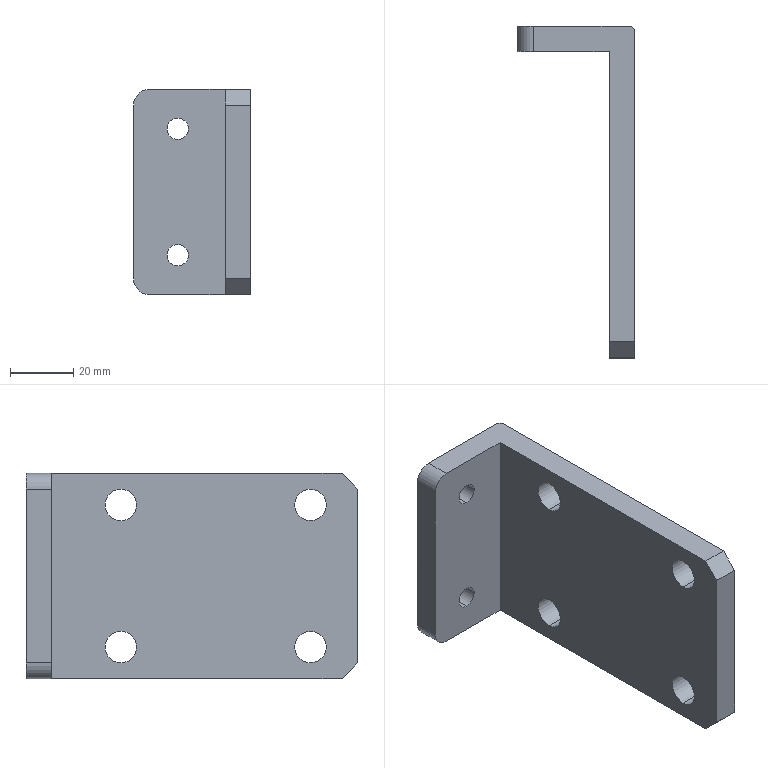Part | NX | features BREP 1 | 1 solid | 25 faces | box 37 x 105 x 65 mm | volume 66267 mm3 | cylinder 14 | plane 11 | commonest cylinder face diameters 10 x10 6.8 x4
STEP:
#1=CARTESIAN_POINT('',(0.,-30.,5.));
#2=VERTEX_POINT('',#1);
#3=CARTESIAN_POINT('',(0.,-30.,15.));
#4=VERTEX_POINT('',#3);
#5=CARTESIAN_POINT('',(0.,-30.,10.));
#6=DIRECTION('',(-1.,0.,0.));
#7=DIRECTION('',(0.,0.,1.));
#8=AXIS2_PLACEMENT_3D('',#5,#6,#7);
#9=CIRCLE('',#8,5.);
#10=EDGE_CURVE('',#2,#4,#9,.T.);
#11=ORIENTED_EDGE('',*,*,#10,.F.);
#12=CARTESIAN_POINT('',(-8.,-30.,5.));
#13=VERTEX_POINT('',#12);
#14=CARTESIAN_POINT('',(-8.,-30.,5.));
#15=DIRECTION('',(-1.,0.,0.));
#16=VECTOR('',#15,1000.);
#17=LINE('',#14,#16);
#18=EDGE_CURVE('',#13,#2,#17,.F.);
#19=ORIENTED_EDGE('',*,*,#18,.F.);
#20=CARTESIAN_POINT('',(-8.,-30.,15.));
#21=VERTEX_POINT('',#20);
#22=CARTESIAN_POINT('',(-8.,-30.,10.));
#23=DIRECTION('',(-1.,0.,0.));
#24=DIRECTION('',(0.,0.,1.));
#25=AXIS2_PLACEMENT_3D('',#22,#23,#24);
#26=CIRCLE('',#25,5.);
#27=EDGE_CURVE('',#13,#21,#26,.T.);
#28=ORIENTED_EDGE('',*,*,#27,.T.);
#29=CARTESIAN_POINT('',(-8.,-30.,15.));
#30=DIRECTION('',(-1.,0.,0.));
#31=VECTOR('',#30,1000.);
#32=LINE('',#29,#31);
#33=EDGE_CURVE('',#21,#4,#32,.F.);
#34=ORIENTED_EDGE('',*,*,#33,.T.);
#35=EDGE_LOOP('',(#11,#19,#28,#34));
#36=FACE_BOUND('',#35,.T.);
#37=CARTESIAN_POINT('',(-8.,-30.,10.));
#38=DIRECTION('',(-1.,0.,0.));
#39=DIRECTION('',(0.,0.,1.));
#40=AXIS2_PLACEMENT_3D('',#37,#38,#39);
#41=CYLINDRICAL_SURFACE('',#40,5.);
#42=ADVANCED_FACE('',(#36),#41,.F.);
#43=CARTESIAN_POINT('',(0.,-90.,50.));
#44=VERTEX_POINT('',#43);
#45=CARTESIAN_POINT('',(0.,-90.,60.));
#46=VERTEX_POINT('',#45);
#47=CARTESIAN_POINT('',(0.,-90.,55.));
#48=DIRECTION('',(-1.,0.,0.));
#49=DIRECTION('',(0.,0.,1.));
#50=AXIS2_PLACEMENT_3D('',#47,#48,#49);
#51=CIRCLE('',#50,5.);
#52=EDGE_CURVE('',#44,#46,#51,.T.);
#53=ORIENTED_EDGE('',*,*,#52,.F.);
#54=CARTESIAN_POINT('',(-8.,-90.,50.));
#55=VERTEX_POINT('',#54);
#56=CARTESIAN_POINT('',(-8.,-90.,50.));
#57=DIRECTION('',(-1.,0.,0.));
#58=VECTOR('',#57,1000.);
#59=LINE('',#56,#58);
#60=EDGE_CURVE('',#55,#44,#59,.F.);
#61=ORIENTED_EDGE('',*,*,#60,.F.);
#62=CARTESIAN_POINT('',(-8.,-90.,60.));
#63=VERTEX_POINT('',#62);
#64=CARTESIAN_POINT('',(-8.,-90.,55.));
#65=DIRECTION('',(-1.,0.,0.));
#66=DIRECTION('',(0.,0.,1.));
#67=AXIS2_PLACEMENT_3D('',#64,#65,#66);
#68=CIRCLE('',#67,5.);
#69=EDGE_CURVE('',#55,#63,#68,.T.);
#70=ORIENTED_EDGE('',*,*,#69,.T.);
#71=CARTESIAN_POINT('',(-8.,-90.,60.));
#72=DIRECTION('',(-1.,0.,0.));
#73=VECTOR('',#72,1000.);
#74=LINE('',#71,#73);
#75=EDGE_CURVE('',#63,#46,#74,.F.);
#76=ORIENTED_EDGE('',*,*,#75,.T.);
#77=EDGE_LOOP('',(#53,#61,#70,#76));
#78=FACE_BOUND('',#77,.T.);
#79=CARTESIAN_POINT('',(-8.,-90.,55.));
#80=DIRECTION('',(-1.,0.,0.));
#81=DIRECTION('',(0.,0.,1.));
#82=AXIS2_PLACEMENT_3D('',#79,#80,#81);
#83=CYLINDRICAL_SURFACE('',#82,5.);
#84=ADVANCED_FACE('',(#78),#83,.F.);
#85=CARTESIAN_POINT('',(0.,-90.,5.));
#86=VERTEX_POINT('',#85);
#87=CARTESIAN_POINT('',(0.,-90.,15.));
#88=VERTEX_POINT('',#87);
#89=CARTESIAN_POINT('',(0.,-90.,10.));
#90=DIRECTION('',(-1.,0.,0.));
#91=DIRECTION('',(0.,0.,1.));
#92=AXIS2_PLACEMENT_3D('',#89,#90,#91);
#93=CIRCLE('',#92,5.);
#94=EDGE_CURVE('',#86,#88,#93,.T.);
#95=ORIENTED_EDGE('',*,*,#94,.F.);
#96=CARTESIAN_POINT('',(-8.,-90.,5.));
#97=VERTEX_POINT('',#96);
#98=CARTESIAN_POINT('',(-8.,-90.,5.));
#99=DIRECTION('',(-1.,0.,0.));
#100=VECTOR('',#99,1000.);
#101=LINE('',#98,#100);
#102=EDGE_CURVE('',#97,#86,#101,.F.);
#103=ORIENTED_EDGE('',*,*,#102,.F.);
#104=CARTESIAN_POINT('',(-8.,-90.,15.));
#105=VERTEX_POINT('',#104);
#106=CARTESIAN_POINT('',(-8.,-90.,10.));
#107=DIRECTION('',(-1.,0.,0.));
#108=DIRECTION('',(0.,0.,1.));
#109=AXIS2_PLACEMENT_3D('',#106,#107,#108);
#110=CIRCLE('',#109,5.);
#111=EDGE_CURVE('',#97,#105,#110,.T.);
#112=ORIENTED_EDGE('',*,*,#111,.T.);
#113=CARTESIAN_POINT('',(-8.,-90.,15.));
#114=DIRECTION('',(-1.,0.,0.));
#115=VECTOR('',#114,1000.);
#116=LINE('',#113,#115);
#117=EDGE_CURVE('',#105,#88,#116,.F.);
#118=ORIENTED_EDGE('',*,*,#117,.T.);
#119=EDGE_LOOP('',(#95,#103,#112,#118));
#120=FACE_BOUND('',#119,.T.);
#121=CARTESIAN_POINT('',(-8.,-90.,10.));
#122=DIRECTION('',(-1.,0.,0.));
#123=DIRECTION('',(0.,0.,1.));
#124=AXIS2_PLACEMENT_3D('',#121,#122,#123);
#125=CYLINDRICAL_SURFACE('',#124,5.);
#126=ADVANCED_FACE('',(#120),#125,.F.);
#127=CARTESIAN_POINT('',(0.,-30.,50.));
#128=VERTEX_POINT('',#127);
#129=CARTESIAN_POINT('',(0.,-30.,60.));
#130=VERTEX_POINT('',#129);
#131=CARTESIAN_POINT('',(0.,-30.,55.));
#132=DIRECTION('',(-1.,0.,0.));
#133=DIRECTION('',(0.,0.,1.));
#134=AXIS2_PLACEMENT_3D('',#131,#132,#133);
#135=CIRCLE('',#134,5.);
#136=EDGE_CURVE('',#128,#130,#135,.T.);
#137=ORIENTED_EDGE('',*,*,#136,.F.);
#138=CARTESIAN_POINT('',(-8.,-30.,50.));
#139=VERTEX_POINT('',#138);
#140=CARTESIAN_POINT('',(-8.,-30.,50.));
#141=DIRECTION('',(-1.,0.,0.));
#142=VECTOR('',#141,1000.);
#143=LINE('',#140,#142);
#144=EDGE_CURVE('',#139,#128,#143,.F.);
#145=ORIENTED_EDGE('',*,*,#144,.F.);
#146=CARTESIAN_POINT('',(-8.,-30.,60.));
#147=VERTEX_POINT('',#146);
#148=CARTESIAN_POINT('',(-8.,-30.,55.));
#149=DIRECTION('',(-1.,0.,0.));
#150=DIRECTION('',(0.,0.,1.));
#151=AXIS2_PLACEMENT_3D('',#148,#149,#150);
#152=CIRCLE('',#151,5.);
#153=EDGE_CURVE('',#139,#147,#152,.T.);
#154=ORIENTED_EDGE('',*,*,#153,.T.);
#155=CARTESIAN_POINT('',(-8.,-30.,60.));
#156=DIRECTION('',(-1.,0.,0.));
#157=VECTOR('',#156,1000.);
#158=LINE('',#155,#157);
#159=EDGE_CURVE('',#147,#130,#158,.F.);
#160=ORIENTED_EDGE('',*,*,#159,.T.);
#161=EDGE_LOOP('',(#137,#145,#154,#160));
#162=FACE_BOUND('',#161,.T.);
#163=CARTESIAN_POINT('',(-8.,-30.,55.));
#164=DIRECTION('',(-1.,0.,0.));
#165=DIRECTION('',(0.,0.,1.));
#166=AXIS2_PLACEMENT_3D('',#163,#164,#165);
#167=CYLINDRICAL_SURFACE('',#166,5.);
#168=ADVANCED_FACE('',(#162),#167,.F.);
#169=CARTESIAN_POINT('',(-23.,-8.,9.1));
#170=VERTEX_POINT('',#169);
#171=CARTESIAN_POINT('',(-23.,-8.,15.9));
#172=VERTEX_POINT('',#171);
#173=CARTESIAN_POINT('',(-23.,-8.,12.5));
#174=DIRECTION('',(0.,1.,0.));
#175=DIRECTION('',(0.,0.,1.));
#176=AXIS2_PLACEMENT_3D('',#173,#174,#175);
#177=CIRCLE('',#176,3.4);
#178=EDGE_CURVE('',#170,#172,#177,.T.);
#179=ORIENTED_EDGE('',*,*,#178,.F.);
#180=CARTESIAN_POINT('',(-23.,0.,9.1));
#181=VERTEX_POINT('',#180);
#182=CARTESIAN_POINT('',(-23.,0.,9.1));
#183=DIRECTION('',(0.,1.,0.));
#184=VECTOR('',#183,1000.);
#185=LINE('',#182,#184);
#186=EDGE_CURVE('',#181,#170,#185,.F.);
#187=ORIENTED_EDGE('',*,*,#186,.F.);
#188=CARTESIAN_POINT('',(-23.,0.,15.9));
#189=VERTEX_POINT('',#188);
#190=CARTESIAN_POINT('',(-23.,0.,12.5));
#191=DIRECTION('',(0.,1.,0.));
#192=DIRECTION('',(0.,0.,1.));
#193=AXIS2_PLACEMENT_3D('',#190,#191,#192);
#194=CIRCLE('',#193,3.4);
#195=EDGE_CURVE('',#181,#189,#194,.T.);
#196=ORIENTED_EDGE('',*,*,#195,.T.);
#197=CARTESIAN_POINT('',(-23.,0.,15.9));
#198=DIRECTION('',(0.,1.,0.));
#199=VECTOR('',#198,1000.);
#200=LINE('',#197,#199);
#201=EDGE_CURVE('',#189,#172,#200,.F.);
#202=ORIENTED_EDGE('',*,*,#201,.T.);
#203=EDGE_LOOP('',(#179,#187,#196,#202));
#204=FACE_BOUND('',#203,.T.);
#205=CARTESIAN_POINT('',(-23.,0.,12.5));
#206=DIRECTION('',(0.,1.,0.));
#207=DIRECTION('',(0.,0.,1.));
#208=AXIS2_PLACEMENT_3D('',#205,#206,#207);
#209=CYLINDRICAL_SURFACE('',#208,3.4);
#210=ADVANCED_FACE('',(#204),#209,.F.);
#211=CARTESIAN_POINT('',(-23.,-8.,49.1));
#212=VERTEX_POINT('',#211);
#213=CARTESIAN_POINT('',(-23.,-8.,55.9));
#214=VERTEX_POINT('',#213);
#215=CARTESIAN_POINT('',(-23.,-8.,52.5));
#216=DIRECTION('',(0.,1.,0.));
#217=DIRECTION('',(0.,0.,1.));
#218=AXIS2_PLACEMENT_3D('',#215,#216,#217);
#219=CIRCLE('',#218,3.4);
#220=EDGE_CURVE('',#212,#214,#219,.T.);
#221=ORIENTED_EDGE('',*,*,#220,.F.);
#222=CARTESIAN_POINT('',(-23.,0.,49.1));
#223=VERTEX_POINT('',#222);
#224=CARTESIAN_POINT('',(-23.,0.,49.1));
#225=DIRECTION('',(0.,1.,0.));
#226=VECTOR('',#225,1000.);
#227=LINE('',#224,#226);
#228=EDGE_CURVE('',#223,#212,#227,.F.);
#229=ORIENTED_EDGE('',*,*,#228,.F.);
#230=CARTESIAN_POINT('',(-23.,0.,55.9));
#231=VERTEX_POINT('',#230);
#232=CARTESIAN_POINT('',(-23.,0.,52.5));
#233=DIRECTION('',(0.,1.,0.));
#234=DIRECTION('',(0.,0.,1.));
#235=AXIS2_PLACEMENT_3D('',#232,#233,#234);
#236=CIRCLE('',#235,3.4);
#237=EDGE_CURVE('',#223,#231,#236,.T.);
#238=ORIENTED_EDGE('',*,*,#237,.T.);
#239=CARTESIAN_POINT('',(-23.,0.,55.9));
#240=DIRECTION('',(0.,1.,0.));
#241=VECTOR('',#240,1000.);
#242=LINE('',#239,#241);
#243=EDGE_CURVE('',#231,#214,#242,.F.);
#244=ORIENTED_EDGE('',*,*,#243,.T.);
#245=EDGE_LOOP('',(#221,#229,#238,#244));
#246=FACE_BOUND('',#245,.T.);
#247=CARTESIAN_POINT('',(-23.,0.,52.5));
#248=DIRECTION('',(0.,1.,0.));
#249=DIRECTION('',(0.,0.,1.));
#250=AXIS2_PLACEMENT_3D('',#247,#248,#249);
#251=CYLINDRICAL_SURFACE('',#250,3.4);
#252=ADVANCED_FACE('',(#246),#251,.F.);
#253=CARTESIAN_POINT('',(-8.,-105.,60.));
#254=VERTEX_POINT('',#253);
#255=CARTESIAN_POINT('',(-8.,-105.,5.));
#256=VERTEX_POINT('',#255);
#257=CARTESIAN_POINT('',(-8.,-105.,65.));
#258=DIRECTION('',(0.,0.,-1.));
#259=VECTOR('',#258,1000.);
#260=LINE('',#257,#259);
#261=EDGE_CURVE('',#254,#256,#260,.T.);
#262=ORIENTED_EDGE('',*,*,#261,.F.);
#263=CARTESIAN_POINT('',(-8.,-100.,65.));
#264=VERTEX_POINT('',#263);
#265=CARTESIAN_POINT('',(-8.,-100.,65.));
#266=DIRECTION('',(0.,0.7071,0.7071));
#267=VECTOR('',#266,1000.);
#268=LINE('',#265,#267);
#269=EDGE_CURVE('',#254,#264,#268,.T.);
#270=ORIENTED_EDGE('',*,*,#269,.T.);
#271=CARTESIAN_POINT('',(-8.,-8.,65.));
#272=VERTEX_POINT('',#271);
#273=CARTESIAN_POINT('',(-8.,-8.,65.));
#274=DIRECTION('',(0.,-1.,0.));
#275=VECTOR('',#274,1000.);
#276=LINE('',#273,#275);
#277=EDGE_CURVE('',#272,#264,#276,.T.);
#278=ORIENTED_EDGE('',*,*,#277,.F.);
#279=CARTESIAN_POINT('',(-8.,-8.,0.));
#280=VERTEX_POINT('',#279);
#281=CARTESIAN_POINT('',(-8.,-8.,65.));
#282=DIRECTION('',(0.,0.,-1.));
#283=VECTOR('',#282,1000.);
#284=LINE('',#281,#283);
#285=EDGE_CURVE('',#272,#280,#284,.T.);
#286=ORIENTED_EDGE('',*,*,#285,.T.);
#287=CARTESIAN_POINT('',(-8.,-100.,0.));
#288=VERTEX_POINT('',#287);
#289=CARTESIAN_POINT('',(-8.,-8.,0.));
#290=DIRECTION('',(0.,-1.,0.));
#291=VECTOR('',#290,1000.);
#292=LINE('',#289,#291);
#293=EDGE_CURVE('',#280,#288,#292,.T.);
#294=ORIENTED_EDGE('',*,*,#293,.T.);
#295=CARTESIAN_POINT('',(-8.,-105.,5.));
#296=DIRECTION('',(0.,-0.7071,0.7071));
#297=VECTOR('',#296,1000.);
#298=LINE('',#295,#297);
#299=EDGE_CURVE('',#288,#256,#298,.T.);
#300=ORIENTED_EDGE('',*,*,#299,.T.);
#301=EDGE_LOOP('',(#262,#270,#278,#286,#294,#300));
#302=FACE_BOUND('',#301,.T.);
#303=CARTESIAN_POINT('',(-8.,-30.,10.));
#304=DIRECTION('',(-1.,0.,0.));
#305=DIRECTION('',(0.,0.,1.));
#306=AXIS2_PLACEMENT_3D('',#303,#304,#305);
#307=CIRCLE('',#306,5.);
#308=EDGE_CURVE('',#21,#13,#307,.T.);
#309=ORIENTED_EDGE('',*,*,#308,.F.);
#310=ORIENTED_EDGE('',*,*,#27,.F.);
#311=EDGE_LOOP('',(#309,#310));
#312=FACE_BOUND('',#311,.T.);
#313=CARTESIAN_POINT('',(-8.,-90.,55.));
#314=DIRECTION('',(-1.,0.,0.));
#315=DIRECTION('',(0.,0.,1.));
#316=AXIS2_PLACEMENT_3D('',#313,#314,#315);
#317=CIRCLE('',#316,5.);
#318=EDGE_CURVE('',#63,#55,#317,.T.);
#319=ORIENTED_EDGE('',*,*,#318,.F.);
#320=ORIENTED_EDGE('',*,*,#69,.F.);
#321=EDGE_LOOP('',(#319,#320));
#322=FACE_BOUND('',#321,.T.);
#323=CARTESIAN_POINT('',(-8.,-30.,55.));
#324=DIRECTION('',(-1.,0.,0.));
#325=DIRECTION('',(0.,0.,1.));
#326=AXIS2_PLACEMENT_3D('',#323,#324,#325);
#327=CIRCLE('',#326,5.);
#328=EDGE_CURVE('',#147,#139,#327,.T.);
#329=ORIENTED_EDGE('',*,*,#328,.F.);
#330=ORIENTED_EDGE('',*,*,#153,.F.);
#331=EDGE_LOOP('',(#329,#330));
#332=FACE_BOUND('',#331,.T.);
#333=CARTESIAN_POINT('',(-8.,-90.,10.));
#334=DIRECTION('',(-1.,0.,0.));
#335=DIRECTION('',(0.,0.,1.));
#336=AXIS2_PLACEMENT_3D('',#333,#334,#335);
#337=CIRCLE('',#336,5.);
#338=EDGE_CURVE('',#105,#97,#337,.T.);
#339=ORIENTED_EDGE('',*,*,#338,.F.);
#340=ORIENTED_EDGE('',*,*,#111,.F.);
#341=EDGE_LOOP('',(#339,#340));
#342=FACE_BOUND('',#341,.T.);
#343=CARTESIAN_POINT('',(-8.,-8.,65.));
#344=DIRECTION('',(1.,0.,0.));
#345=DIRECTION('',(0.,1.,0.));
#346=AXIS2_PLACEMENT_3D('',#343,#344,#345);
#347=PLANE('',#346);
#348=ADVANCED_FACE('',(#302,#312,#322,#332,#342),#347,.F.);
#349=CARTESIAN_POINT('',(0.,-100.,0.));
#350=VERTEX_POINT('',#349);
#351=CARTESIAN_POINT('',(0.,-1.,0.));
#352=VERTEX_POINT('',#351);
#353=CARTESIAN_POINT('',(0.,-105.,0.));
#354=DIRECTION('',(0.,1.,0.));
#355=VECTOR('',#354,1000.);
#356=LINE('',#353,#355);
#357=EDGE_CURVE('',#350,#352,#356,.T.);
#358=ORIENTED_EDGE('',*,*,#357,.T.);
#359=CARTESIAN_POINT('',(0.,-1.,65.));
#360=VERTEX_POINT('',#359);
#361=CARTESIAN_POINT('',(0.,-1.,65.));
#362=DIRECTION('',(0.,0.,1.));
#363=VECTOR('',#362,1000.);
#364=LINE('',#361,#363);
#365=EDGE_CURVE('',#352,#360,#364,.T.);
#366=ORIENTED_EDGE('',*,*,#365,.T.);
#367=CARTESIAN_POINT('',(0.,-100.,65.));
#368=VERTEX_POINT('',#367);
#369=CARTESIAN_POINT('',(0.,-105.,65.));
#370=DIRECTION('',(0.,1.,0.));
#371=VECTOR('',#370,1000.);
#372=LINE('',#369,#371);
#373=EDGE_CURVE('',#368,#360,#372,.T.);
#374=ORIENTED_EDGE('',*,*,#373,.F.);
#375=CARTESIAN_POINT('',(0.,-105.,60.));
#376=VERTEX_POINT('',#375);
#377=CARTESIAN_POINT('',(0.,-100.,65.));
#378=DIRECTION('',(0.,-0.7071,-0.7071));
#379=VECTOR('',#378,1000.);
#380=LINE('',#377,#379);
#381=EDGE_CURVE('',#368,#376,#380,.T.);
#382=ORIENTED_EDGE('',*,*,#381,.T.);
#383=CARTESIAN_POINT('',(0.,-105.,5.));
#384=VERTEX_POINT('',#383);
#385=CARTESIAN_POINT('',(0.,-105.,65.));
#386=DIRECTION('',(0.,0.,-1.));
#387=VECTOR('',#386,1000.);
#388=LINE('',#385,#387);
#389=EDGE_CURVE('',#376,#384,#388,.T.);
#390=ORIENTED_EDGE('',*,*,#389,.T.);
#391=CARTESIAN_POINT('',(0.,-105.,5.));
#392=DIRECTION('',(0.,0.7071,-0.7071));
#393=VECTOR('',#392,1000.);
#394=LINE('',#391,#393);
#395=EDGE_CURVE('',#384,#350,#394,.T.);
#396=ORIENTED_EDGE('',*,*,#395,.T.);
#397=EDGE_LOOP('',(#358,#366,#374,#382,#390,#396));
#398=FACE_BOUND('',#397,.T.);
#399=CARTESIAN_POINT('',(0.,-30.,10.));
#400=DIRECTION('',(-1.,0.,0.));
#401=DIRECTION('',(0.,0.,1.));
#402=AXIS2_PLACEMENT_3D('',#399,#400,#401);
#403=CIRCLE('',#402,5.);
#404=EDGE_CURVE('',#4,#2,#403,.T.);
#405=ORIENTED_EDGE('',*,*,#404,.T.);
#406=ORIENTED_EDGE('',*,*,#10,.T.);
#407=EDGE_LOOP('',(#405,#406));
#408=FACE_BOUND('',#407,.T.);
#409=CARTESIAN_POINT('',(0.,-90.,55.));
#410=DIRECTION('',(-1.,0.,0.));
#411=DIRECTION('',(0.,0.,1.));
#412=AXIS2_PLACEMENT_3D('',#409,#410,#411);
#413=CIRCLE('',#412,5.);
#414=EDGE_CURVE('',#46,#44,#413,.T.);
#415=ORIENTED_EDGE('',*,*,#414,.T.);
#416=ORIENTED_EDGE('',*,*,#52,.T.);
#417=EDGE_LOOP('',(#415,#416));
#418=FACE_BOUND('',#417,.T.);
#419=CARTESIAN_POINT('',(0.,-90.,10.));
#420=DIRECTION('',(-1.,0.,0.));
#421=DIRECTION('',(0.,0.,1.));
#422=AXIS2_PLACEMENT_3D('',#419,#420,#421);
#423=CIRCLE('',#422,5.);
#424=EDGE_CURVE('',#88,#86,#423,.T.);
#425=ORIENTED_EDGE('',*,*,#424,.T.);
#426=ORIENTED_EDGE('',*,*,#94,.T.);
#427=EDGE_LOOP('',(#425,#426));
#428=FACE_BOUND('',#427,.T.);
#429=CARTESIAN_POINT('',(0.,-30.,55.));
#430=DIRECTION('',(-1.,0.,0.));
#431=DIRECTION('',(0.,0.,1.));
#432=AXIS2_PLACEMENT_3D('',#429,#430,#431);
#433=CIRCLE('',#432,5.);
#434=EDGE_CURVE('',#130,#128,#433,.T.);
#435=ORIENTED_EDGE('',*,*,#434,.T.);
#436=ORIENTED_EDGE('',*,*,#136,.T.);
#437=EDGE_LOOP('',(#435,#436));
#438=FACE_BOUND('',#437,.T.);
#439=CARTESIAN_POINT('',(0.,-105.,65.));
#440=DIRECTION('',(-1.,0.,0.));
#441=DIRECTION('',(0.,1.,0.));
#442=AXIS2_PLACEMENT_3D('',#439,#440,#441);
#443=PLANE('',#442);
#444=ADVANCED_FACE('',(#398,#408,#418,#428,#438),#443,.F.);
#445=CARTESIAN_POINT('',(-1.,0.,65.));
#446=VERTEX_POINT('',#445);
#447=CARTESIAN_POINT('',(-32.,0.,65.));
#448=VERTEX_POINT('',#447);
#449=CARTESIAN_POINT('',(0.,0.,65.));
#450=DIRECTION('',(-1.,0.,0.));
#451=VECTOR('',#450,1000.);
#452=LINE('',#449,#451);
#453=EDGE_CURVE('',#446,#448,#452,.T.);
#454=ORIENTED_EDGE('',*,*,#453,.F.);
#455=CARTESIAN_POINT('',(-1.,0.,0.));
#456=VERTEX_POINT('',#455);
#457=CARTESIAN_POINT('',(-1.,0.,65.));
#458=DIRECTION('',(0.,0.,-1.));
#459=VECTOR('',#458,1000.);
#460=LINE('',#457,#459);
#461=EDGE_CURVE('',#446,#456,#460,.T.);
#462=ORIENTED_EDGE('',*,*,#461,.T.);
#463=CARTESIAN_POINT('',(-32.,0.,0.));
#464=VERTEX_POINT('',#463);
#465=CARTESIAN_POINT('',(0.,0.,0.));
#466=DIRECTION('',(-1.,0.,0.));
#467=VECTOR('',#466,1000.);
#468=LINE('',#465,#467);
#469=EDGE_CURVE('',#456,#464,#468,.T.);
#470=ORIENTED_EDGE('',*,*,#469,.T.);
#471=CARTESIAN_POINT('',(-37.,0.,5.));
#472=VERTEX_POINT('',#471);
#473=CARTESIAN_POINT('',(-32.,0.,5.));
#474=DIRECTION('',(0.,1.,0.));
#475=DIRECTION('',(1.,0.,0.));
#476=AXIS2_PLACEMENT_3D('',#473,#474,#475);
#477=CIRCLE('',#476,5.);
#478=EDGE_CURVE('',#464,#472,#477,.T.);
#479=ORIENTED_EDGE('',*,*,#478,.T.);
#480=CARTESIAN_POINT('',(-37.,0.,60.));
#481=VERTEX_POINT('',#480);
#482=CARTESIAN_POINT('',(-37.,0.,65.));
#483=DIRECTION('',(0.,0.,-1.));
#484=VECTOR('',#483,1000.);
#485=LINE('',#482,#484);
#486=EDGE_CURVE('',#481,#472,#485,.T.);
#487=ORIENTED_EDGE('',*,*,#486,.F.);
#488=CARTESIAN_POINT('',(-32.,0.,60.));
#489=DIRECTION('',(0.,1.,0.));
#490=DIRECTION('',(1.,0.,0.));
#491=AXIS2_PLACEMENT_3D('',#488,#489,#490);
#492=CIRCLE('',#491,5.);
#493=EDGE_CURVE('',#481,#448,#492,.T.);
#494=ORIENTED_EDGE('',*,*,#493,.T.);
#495=EDGE_LOOP('',(#454,#462,#470,#479,#487,#494));
#496=FACE_BOUND('',#495,.T.);
#497=CARTESIAN_POINT('',(-23.,0.,12.5));
#498=DIRECTION('',(0.,1.,0.));
#499=DIRECTION('',(0.,0.,1.));
#500=AXIS2_PLACEMENT_3D('',#497,#498,#499);
#501=CIRCLE('',#500,3.4);
#502=EDGE_CURVE('',#189,#181,#501,.T.);
#503=ORIENTED_EDGE('',*,*,#502,.F.);
#504=ORIENTED_EDGE('',*,*,#195,.F.);
#505=EDGE_LOOP('',(#503,#504));
#506=FACE_BOUND('',#505,.T.);
#507=CARTESIAN_POINT('',(-23.,0.,52.5));
#508=DIRECTION('',(0.,1.,0.));
#509=DIRECTION('',(0.,0.,1.));
#510=AXIS2_PLACEMENT_3D('',#507,#508,#509);
#511=CIRCLE('',#510,3.4);
#512=EDGE_CURVE('',#231,#223,#511,.T.);
#513=ORIENTED_EDGE('',*,*,#512,.F.);
#514=ORIENTED_EDGE('',*,*,#237,.F.);
#515=EDGE_LOOP('',(#513,#514));
#516=FACE_BOUND('',#515,.T.);
#517=CARTESIAN_POINT('',(0.,0.,65.));
#518=DIRECTION('',(0.,-1.,0.));
#519=DIRECTION('',(0.,0.,-1.));
#520=AXIS2_PLACEMENT_3D('',#517,#518,#519);
#521=PLANE('',#520);
#522=ADVANCED_FACE('',(#496,#506,#516),#521,.F.);
#523=ORIENTED_EDGE('',*,*,#486,.T.);
#524=CARTESIAN_POINT('',(-37.,-8.,5.));
#525=VERTEX_POINT('',#524);
#526=CARTESIAN_POINT('',(-37.,0.,5.));
#527=DIRECTION('',(0.,-1.,0.));
#528=VECTOR('',#527,1000.);
#529=LINE('',#526,#528);
#530=EDGE_CURVE('',#472,#525,#529,.T.);
#531=ORIENTED_EDGE('',*,*,#530,.T.);
#532=CARTESIAN_POINT('',(-37.,-8.,60.));
#533=VERTEX_POINT('',#532);
#534=CARTESIAN_POINT('',(-37.,-8.,65.));
#535=DIRECTION('',(0.,0.,-1.));
#536=VECTOR('',#535,1000.);
#537=LINE('',#534,#536);
#538=EDGE_CURVE('',#533,#525,#537,.T.);
#539=ORIENTED_EDGE('',*,*,#538,.F.);
#540=CARTESIAN_POINT('',(-37.,0.,60.));
#541=DIRECTION('',(0.,1.,0.));
#542=VECTOR('',#541,1000.);
#543=LINE('',#540,#542);
#544=EDGE_CURVE('',#533,#481,#543,.T.);
#545=ORIENTED_EDGE('',*,*,#544,.T.);
#546=EDGE_LOOP('',(#523,#531,#539,#545));
#547=FACE_BOUND('',#546,.T.);
#548=CARTESIAN_POINT('',(-37.,0.,65.));
#549=DIRECTION('',(1.,0.,0.));
#550=DIRECTION('',(0.,1.,0.));
#551=AXIS2_PLACEMENT_3D('',#548,#549,#550);
#552=PLANE('',#551);
#553=ADVANCED_FACE('',(#547),#552,.F.);
#554=ORIENTED_EDGE('',*,*,#538,.T.);
#555=CARTESIAN_POINT('',(-32.,-8.,0.));
#556=VERTEX_POINT('',#555);
#557=CARTESIAN_POINT('',(-32.,-8.,5.));
#558=DIRECTION('',(0.,-1.,0.));
#559=DIRECTION('',(0.,0.,1.));
#560=AXIS2_PLACEMENT_3D('',#557,#558,#559);
#561=CIRCLE('',#560,5.);
#562=EDGE_CURVE('',#525,#556,#561,.T.);
#563=ORIENTED_EDGE('',*,*,#562,.T.);
#564=CARTESIAN_POINT('',(-37.,-8.,0.));
#565=DIRECTION('',(1.,0.,0.));
#566=VECTOR('',#565,1000.);
#567=LINE('',#564,#566);
#568=EDGE_CURVE('',#556,#280,#567,.T.);
#569=ORIENTED_EDGE('',*,*,#568,.T.);
#570=ORIENTED_EDGE('',*,*,#285,.F.);
#571=CARTESIAN_POINT('',(-32.,-8.,65.));
#572=VERTEX_POINT('',#571);
#573=CARTESIAN_POINT('',(-37.,-8.,65.));
#574=DIRECTION('',(1.,0.,0.));
#575=VECTOR('',#574,1000.);
#576=LINE('',#573,#575);
#577=EDGE_CURVE('',#572,#272,#576,.T.);
#578=ORIENTED_EDGE('',*,*,#577,.F.);
#579=CARTESIAN_POINT('',(-32.,-8.,60.));
#580=DIRECTION('',(0.,-1.,0.));
#581=DIRECTION('',(0.,0.,1.));
#582=AXIS2_PLACEMENT_3D('',#579,#580,#581);
#583=CIRCLE('',#582,5.);
#584=EDGE_CURVE('',#572,#533,#583,.T.);
#585=ORIENTED_EDGE('',*,*,#584,.T.);
#586=EDGE_LOOP('',(#554,#563,#569,#570,#578,#585));
#587=FACE_BOUND('',#586,.T.);
#588=CARTESIAN_POINT('',(-23.,-8.,12.5));
#589=DIRECTION('',(0.,1.,0.));
#590=DIRECTION('',(0.,0.,1.));
#591=AXIS2_PLACEMENT_3D('',#588,#589,#590);
#592=CIRCLE('',#591,3.4);
#593=EDGE_CURVE('',#172,#170,#592,.T.);
#594=ORIENTED_EDGE('',*,*,#593,.T.);
#595=ORIENTED_EDGE('',*,*,#178,.T.);
#596=EDGE_LOOP('',(#594,#595));
#597=FACE_BOUND('',#596,.T.);
#598=CARTESIAN_POINT('',(-23.,-8.,52.5));
#599=DIRECTION('',(0.,1.,0.));
#600=DIRECTION('',(0.,0.,1.));
#601=AXIS2_PLACEMENT_3D('',#598,#599,#600);
#602=CIRCLE('',#601,3.4);
#603=EDGE_CURVE('',#214,#212,#602,.T.);
#604=ORIENTED_EDGE('',*,*,#603,.T.);
#605=ORIENTED_EDGE('',*,*,#220,.T.);
#606=EDGE_LOOP('',(#604,#605));
#607=FACE_BOUND('',#606,.T.);
#608=CARTESIAN_POINT('',(-37.,-8.,65.));
#609=DIRECTION('',(0.,1.,0.));
#610=DIRECTION('',(1.,0.,0.));
#611=AXIS2_PLACEMENT_3D('',#608,#609,#610);
#612=PLANE('',#611);
#613=ADVANCED_FACE('',(#587,#597,#607),#612,.F.);
#614=ORIENTED_EDGE('',*,*,#389,.F.);
#615=CARTESIAN_POINT('',(-8.,-105.,60.));
#616=DIRECTION('',(-1.,0.,0.));
#617=VECTOR('',#616,1000.);
#618=LINE('',#615,#617);
#619=EDGE_CURVE('',#376,#254,#618,.T.);
#620=ORIENTED_EDGE('',*,*,#619,.T.);
#621=ORIENTED_EDGE('',*,*,#261,.T.);
#622=CARTESIAN_POINT('',(-8.,-105.,5.));
#623=DIRECTION('',(1.,0.,0.));
#624=VECTOR('',#623,1000.);
#625=LINE('',#622,#624);
#626=EDGE_CURVE('',#256,#384,#625,.T.);
#627=ORIENTED_EDGE('',*,*,#626,.T.);
#628=EDGE_LOOP('',(#614,#620,#621,#627));
#629=FACE_BOUND('',#628,.T.);
#630=CARTESIAN_POINT('',(-8.,-105.,65.));
#631=DIRECTION('',(0.,1.,0.));
#632=DIRECTION('',(1.,0.,0.));
#633=AXIS2_PLACEMENT_3D('',#630,#631,#632);
#634=PLANE('',#633);
#635=ADVANCED_FACE('',(#629),#634,.F.);
#636=ORIENTED_EDGE('',*,*,#373,.T.);
#637=CARTESIAN_POINT('',(-0.5,-0.5,65.));
#638=DIRECTION('',(-0.7071,0.7071,0.));
#639=VECTOR('',#638,1000.);
#640=LINE('',#637,#639);
#641=EDGE_CURVE('',#360,#446,#640,.T.);
#642=ORIENTED_EDGE('',*,*,#641,.T.);
#643=ORIENTED_EDGE('',*,*,#453,.T.);
#644=CARTESIAN_POINT('',(-32.,-8.,65.));
#645=DIRECTION('',(0.,-1.,0.));
#646=VECTOR('',#645,1000.);
#647=LINE('',#644,#646);
#648=EDGE_CURVE('',#448,#572,#647,.T.);
#649=ORIENTED_EDGE('',*,*,#648,.T.);
#650=ORIENTED_EDGE('',*,*,#577,.T.);
#651=ORIENTED_EDGE('',*,*,#277,.T.);
#652=CARTESIAN_POINT('',(0.,-100.,65.));
#653=DIRECTION('',(1.,0.,0.));
#654=VECTOR('',#653,1000.);
#655=LINE('',#652,#654);
#656=EDGE_CURVE('',#264,#368,#655,.T.);
#657=ORIENTED_EDGE('',*,*,#656,.T.);
#658=EDGE_LOOP('',(#636,#642,#643,#649,#650,#651,#657));
#659=FACE_BOUND('',#658,.T.);
#660=CARTESIAN_POINT('',(0.,0.,65.));
#661=DIRECTION('',(0.,0.,1.));
#662=DIRECTION('',(1.,0.,0.));
#663=AXIS2_PLACEMENT_3D('',#660,#661,#662);
#664=PLANE('',#663);
#665=ADVANCED_FACE('',(#659),#664,.T.);
#666=ORIENTED_EDGE('',*,*,#469,.F.);
#667=CARTESIAN_POINT('',(-1.,0.,0.));
#668=DIRECTION('',(0.7071,-0.7071,0.));
#669=VECTOR('',#668,1000.);
#670=LINE('',#667,#669);
#671=EDGE_CURVE('',#456,#352,#670,.T.);
#672=ORIENTED_EDGE('',*,*,#671,.T.);
#673=ORIENTED_EDGE('',*,*,#357,.F.);
#674=CARTESIAN_POINT('',(0.,-100.,0.));
#675=DIRECTION('',(-1.,0.,0.));
#676=VECTOR('',#675,1000.);
#677=LINE('',#674,#676);
#678=EDGE_CURVE('',#350,#288,#677,.T.);
#679=ORIENTED_EDGE('',*,*,#678,.T.);
#680=ORIENTED_EDGE('',*,*,#293,.F.);
#681=ORIENTED_EDGE('',*,*,#568,.F.);
#682=CARTESIAN_POINT('',(-32.,0.,0.));
#683=DIRECTION('',(0.,1.,0.));
#684=VECTOR('',#683,1000.);
#685=LINE('',#682,#684);
#686=EDGE_CURVE('',#556,#464,#685,.T.);
#687=ORIENTED_EDGE('',*,*,#686,.T.);
#688=EDGE_LOOP('',(#666,#672,#673,#679,#680,#681,#687));
#689=FACE_BOUND('',#688,.T.);
#690=CARTESIAN_POINT('',(0.,0.,0.));
#691=DIRECTION('',(0.,0.,1.));
#692=DIRECTION('',(1.,0.,0.));
#693=AXIS2_PLACEMENT_3D('',#690,#691,#692);
#694=PLANE('',#693);
#695=ADVANCED_FACE('',(#689),#694,.F.);
#696=ORIENTED_EDGE('',*,*,#478,.F.);
#697=ORIENTED_EDGE('',*,*,#686,.F.);
#698=ORIENTED_EDGE('',*,*,#562,.F.);
#699=ORIENTED_EDGE('',*,*,#530,.F.);
#700=EDGE_LOOP('',(#696,#697,#698,#699));
#701=FACE_BOUND('',#700,.T.);
#702=CARTESIAN_POINT('',(-32.,0.,5.));
#703=DIRECTION('',(0.,-1.,0.));
#704=DIRECTION('',(0.,0.,-1.));
#705=AXIS2_PLACEMENT_3D('',#702,#703,#704);
#706=CYLINDRICAL_SURFACE('',#705,5.);
#707=ADVANCED_FACE('',(#701),#706,.T.);
#708=ORIENTED_EDGE('',*,*,#493,.F.);
#709=ORIENTED_EDGE('',*,*,#544,.F.);
#710=ORIENTED_EDGE('',*,*,#584,.F.);
#711=ORIENTED_EDGE('',*,*,#648,.F.);
#712=EDGE_LOOP('',(#708,#709,#710,#711));
#713=FACE_BOUND('',#712,.T.);
#714=CARTESIAN_POINT('',(-32.,0.,60.));
#715=DIRECTION('',(0.,1.,0.));
#716=DIRECTION('',(0.,0.,1.));
#717=AXIS2_PLACEMENT_3D('',#714,#715,#716);
#718=CYLINDRICAL_SURFACE('',#717,5.);
#719=ADVANCED_FACE('',(#713),#718,.T.);
#720=ORIENTED_EDGE('',*,*,#228,.T.);
#721=ORIENTED_EDGE('',*,*,#603,.F.);
#722=ORIENTED_EDGE('',*,*,#243,.F.);
#723=ORIENTED_EDGE('',*,*,#512,.T.);
#724=EDGE_LOOP('',(#720,#721,#722,#723));
#725=FACE_BOUND('',#724,.T.);
#726=CARTESIAN_POINT('',(-23.,0.,52.5));
#727=DIRECTION('',(0.,1.,0.));
#728=DIRECTION('',(0.,0.,1.));
#729=AXIS2_PLACEMENT_3D('',#726,#727,#728);
#730=CYLINDRICAL_SURFACE('',#729,3.4);
#731=ADVANCED_FACE('',(#725),#730,.F.);
#732=ORIENTED_EDGE('',*,*,#186,.T.);
#733=ORIENTED_EDGE('',*,*,#593,.F.);
#734=ORIENTED_EDGE('',*,*,#201,.F.);
#735=ORIENTED_EDGE('',*,*,#502,.T.);
#736=EDGE_LOOP('',(#732,#733,#734,#735));
#737=FACE_BOUND('',#736,.T.);
#738=CARTESIAN_POINT('',(-23.,0.,12.5));
#739=DIRECTION('',(0.,1.,0.));
#740=DIRECTION('',(0.,0.,1.));
#741=AXIS2_PLACEMENT_3D('',#738,#739,#740);
#742=CYLINDRICAL_SURFACE('',#741,3.4);
#743=ADVANCED_FACE('',(#737),#742,.F.);
#744=ORIENTED_EDGE('',*,*,#144,.T.);
#745=ORIENTED_EDGE('',*,*,#434,.F.);
#746=ORIENTED_EDGE('',*,*,#159,.F.);
#747=ORIENTED_EDGE('',*,*,#328,.T.);
#748=EDGE_LOOP('',(#744,#745,#746,#747));
#749=FACE_BOUND('',#748,.T.);
#750=CARTESIAN_POINT('',(-8.,-30.,55.));
#751=DIRECTION('',(-1.,0.,0.));
#752=DIRECTION('',(0.,0.,1.));
#753=AXIS2_PLACEMENT_3D('',#750,#751,#752);
#754=CYLINDRICAL_SURFACE('',#753,5.);
#755=ADVANCED_FACE('',(#749),#754,.F.);
#756=ORIENTED_EDGE('',*,*,#102,.T.);
#757=ORIENTED_EDGE('',*,*,#424,.F.);
#758=ORIENTED_EDGE('',*,*,#117,.F.);
#759=ORIENTED_EDGE('',*,*,#338,.T.);
#760=EDGE_LOOP('',(#756,#757,#758,#759));
#761=FACE_BOUND('',#760,.T.);
#762=CARTESIAN_POINT('',(-8.,-90.,10.));
#763=DIRECTION('',(-1.,0.,0.));
#764=DIRECTION('',(0.,0.,1.));
#765=AXIS2_PLACEMENT_3D('',#762,#763,#764);
#766=CYLINDRICAL_SURFACE('',#765,5.);
#767=ADVANCED_FACE('',(#761),#766,.F.);
#768=ORIENTED_EDGE('',*,*,#60,.T.);
#769=ORIENTED_EDGE('',*,*,#414,.F.);
#770=ORIENTED_EDGE('',*,*,#75,.F.);
#771=ORIENTED_EDGE('',*,*,#318,.T.);
#772=EDGE_LOOP('',(#768,#769,#770,#771));
#773=FACE_BOUND('',#772,.T.);
#774=CARTESIAN_POINT('',(-8.,-90.,55.));
#775=DIRECTION('',(-1.,0.,0.));
#776=DIRECTION('',(0.,0.,1.));
#777=AXIS2_PLACEMENT_3D('',#774,#775,#776);
#778=CYLINDRICAL_SURFACE('',#777,5.);
#779=ADVANCED_FACE('',(#773),#778,.F.);
#780=ORIENTED_EDGE('',*,*,#18,.T.);
#781=ORIENTED_EDGE('',*,*,#404,.F.);
#782=ORIENTED_EDGE('',*,*,#33,.F.);
#783=ORIENTED_EDGE('',*,*,#308,.T.);
#784=EDGE_LOOP('',(#780,#781,#782,#783));
#785=FACE_BOUND('',#784,.T.);
#786=CARTESIAN_POINT('',(-8.,-30.,10.));
#787=DIRECTION('',(-1.,0.,0.));
#788=DIRECTION('',(0.,0.,1.));
#789=AXIS2_PLACEMENT_3D('',#786,#787,#788);
#790=CYLINDRICAL_SURFACE('',#789,5.);
#791=ADVANCED_FACE('',(#785),#790,.F.);
#792=ORIENTED_EDGE('',*,*,#269,.F.);
#793=ORIENTED_EDGE('',*,*,#619,.F.);
#794=ORIENTED_EDGE('',*,*,#381,.F.);
#795=ORIENTED_EDGE('',*,*,#656,.F.);
#796=EDGE_LOOP('',(#792,#793,#794,#795));
#797=FACE_BOUND('',#796,.T.);
#798=CARTESIAN_POINT('',(0.,-100.,65.));
#799=DIRECTION('',(0.,-0.7071,0.7071));
#800=DIRECTION('',(-1.,0.,0.));
#801=AXIS2_PLACEMENT_3D('',#798,#799,#800);
#802=PLANE('',#801);
#803=ADVANCED_FACE('',(#797),#802,.T.);
#804=ORIENTED_EDGE('',*,*,#299,.F.);
#805=ORIENTED_EDGE('',*,*,#678,.F.);
#806=ORIENTED_EDGE('',*,*,#395,.F.);
#807=ORIENTED_EDGE('',*,*,#626,.F.);
#808=EDGE_LOOP('',(#804,#805,#806,#807));
#809=FACE_BOUND('',#808,.T.);
#810=CARTESIAN_POINT('',(-8.,-105.,5.));
#811=DIRECTION('',(0.,0.7071,0.7071));
#812=DIRECTION('',(1.,0.,0.));
#813=AXIS2_PLACEMENT_3D('',#810,#811,#812);
#814=PLANE('',#813);
#815=ADVANCED_FACE('',(#809),#814,.F.);
#816=ORIENTED_EDGE('',*,*,#641,.F.);
#817=ORIENTED_EDGE('',*,*,#365,.F.);
#818=ORIENTED_EDGE('',*,*,#671,.F.);
#819=ORIENTED_EDGE('',*,*,#461,.F.);
#820=EDGE_LOOP('',(#816,#817,#818,#819));
#821=FACE_BOUND('',#820,.T.);
#822=CARTESIAN_POINT('',(-1.,0.,65.));
#823=DIRECTION('',(-0.7071,-0.7071,0.));
#824=DIRECTION('',(-0.7071,0.7071,0.));
#825=AXIS2_PLACEMENT_3D('',#822,#823,#824);
#826=PLANE('',#825);
#827=ADVANCED_FACE('',(#821),#826,.F.);
#828=CLOSED_SHELL('',(#42,#84,#126,#168,#210,#252,#348,#444,#522,#553,#613,#635,#665,#695,#707,#719,#731,#743,#755,#767,#779,#791,#803,#815,#827));
#829=MANIFOLD_SOLID_BREP('',#828);
#830=(LENGTH_UNIT()NAMED_UNIT(*)SI_UNIT(.MILLI.,.METRE.));
#831=UNCERTAINTY_MEASURE_WITH_UNIT(LENGTH_MEASURE(0.00001),#830,'','');
#832=(NAMED_UNIT(*)PLANE_ANGLE_UNIT()SI_UNIT($,.RADIAN.));
#833=(NAMED_UNIT(*)SI_UNIT($,.STERADIAN.)SOLID_ANGLE_UNIT());
#834=(GEOMETRIC_REPRESENTATION_CONTEXT(3)GLOBAL_UNCERTAINTY_ASSIGNED_CONTEXT((#831))GLOBAL_UNIT_ASSIGNED_CONTEXT((#830,#832,#833))REPRESENTATION_CONTEXT('',''));
#835=ADVANCED_BREP_SHAPE_REPRESENTATION('',(#829),#834);